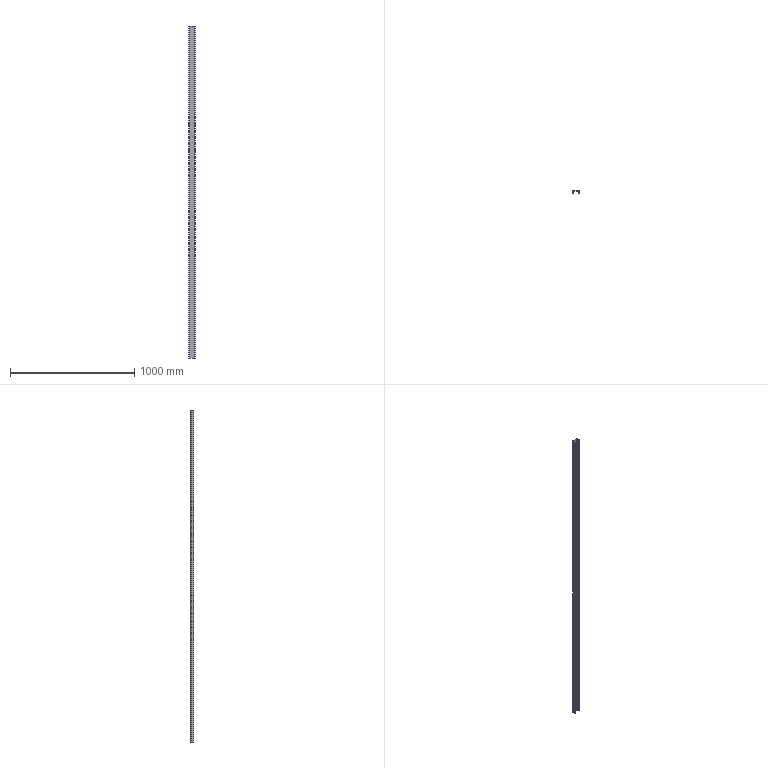Part | STEP file | VD-SYL0380DJ1006_1_2_1-6_STEP | 1 solid | 14 faces | box 50 x 25 x 2672 mm | volume 722540 mm3 | plane 10 | cylinder 4 | commonest cylinder face diameters 6 x2 12 x2
STEP:
#1=CARTESIAN_POINT('',(-19.,20.,1336.));
#2=VERTEX_POINT('',#1);
#3=CARTESIAN_POINT('',(-19.,20.,-1336.));
#4=VERTEX_POINT('',#3);
#5=CARTESIAN_POINT('',(-19.,20.,1336.));
#6=DIRECTION('',(0.,0.,-1.));
#7=VECTOR('',#6,1000.);
#8=LINE('',#5,#7);
#9=EDGE_CURVE('',#2,#4,#8,.T.);
#10=ORIENTED_EDGE('',*,*,#9,.T.);
#11=CARTESIAN_POINT('',(-25.,14.,-1336.));
#12=VERTEX_POINT('',#11);
#13=CARTESIAN_POINT('',(-19.,14.,-1336.));
#14=DIRECTION('',(0.,0.,-1.));
#15=DIRECTION('',(-1.,0.,0.));
#16=AXIS2_PLACEMENT_3D('',#13,#14,#15);
#17=CIRCLE('',#16,6.);
#18=EDGE_CURVE('',#12,#4,#17,.T.);
#19=ORIENTED_EDGE('',*,*,#18,.F.);
#20=CARTESIAN_POINT('',(-25.,14.,1336.));
#21=VERTEX_POINT('',#20);
#22=CARTESIAN_POINT('',(-25.,14.,-1336.));
#23=DIRECTION('',(0.,0.,1.));
#24=VECTOR('',#23,1000.);
#25=LINE('',#22,#24);
#26=EDGE_CURVE('',#12,#21,#25,.T.);
#27=ORIENTED_EDGE('',*,*,#26,.T.);
#28=CARTESIAN_POINT('',(-19.,14.,1336.));
#29=DIRECTION('',(0.,0.,1.));
#30=DIRECTION('',(0.,1.,0.));
#31=AXIS2_PLACEMENT_3D('',#28,#29,#30);
#32=CIRCLE('',#31,6.);
#33=EDGE_CURVE('',#2,#21,#32,.T.);
#34=ORIENTED_EDGE('',*,*,#33,.F.);
#35=EDGE_LOOP('',(#10,#19,#27,#34));
#36=FACE_OUTER_BOUND('',#35,.T.);
#37=CARTESIAN_POINT('',(-19.,14.,4819.219));
#38=DIRECTION('',(0.,0.,-1.));
#39=DIRECTION('',(-1.,0.,0.));
#40=AXIS2_PLACEMENT_3D('',#37,#38,#39);
#41=CYLINDRICAL_SURFACE('',#40,6.);
#42=ADVANCED_FACE('',(#36),#41,.T.);
#43=ORIENTED_EDGE('',*,*,#26,.F.);
#44=CARTESIAN_POINT('',(-25.,-5.,-1336.));
#45=VERTEX_POINT('',#44);
#46=CARTESIAN_POINT('',(-25.,-5.,-1336.));
#47=DIRECTION('',(0.,1.,0.));
#48=VECTOR('',#47,1000.);
#49=LINE('',#46,#48);
#50=EDGE_CURVE('',#45,#12,#49,.T.);
#51=ORIENTED_EDGE('',*,*,#50,.F.);
#52=CARTESIAN_POINT('',(-25.,-5.,1336.));
#53=VERTEX_POINT('',#52);
#54=CARTESIAN_POINT('',(-25.,-5.,1336.));
#55=DIRECTION('',(0.,0.,-1.));
#56=VECTOR('',#55,1000.);
#57=LINE('',#54,#56);
#58=EDGE_CURVE('',#53,#45,#57,.T.);
#59=ORIENTED_EDGE('',*,*,#58,.F.);
#60=CARTESIAN_POINT('',(-25.,14.,1336.));
#61=DIRECTION('',(0.,-1.,0.));
#62=VECTOR('',#61,1000.);
#63=LINE('',#60,#62);
#64=EDGE_CURVE('',#21,#53,#63,.T.);
#65=ORIENTED_EDGE('',*,*,#64,.F.);
#66=EDGE_LOOP('',(#43,#51,#59,#65));
#67=FACE_OUTER_BOUND('',#66,.T.);
#68=CARTESIAN_POINT('',(-25.,20.,-1336.));
#69=DIRECTION('',(-1.,0.,0.));
#70=DIRECTION('',(0.,0.,1.));
#71=AXIS2_PLACEMENT_3D('',#68,#69,#70);
#72=PLANE('',#71);
#73=ADVANCED_FACE('',(#67),#72,.T.);
#74=ORIENTED_EDGE('',*,*,#58,.T.);
#75=CARTESIAN_POINT('',(-22.,-5.,-1336.));
#76=VERTEX_POINT('',#75);
#77=CARTESIAN_POINT('',(-22.,-5.,-1336.));
#78=DIRECTION('',(-1.,0.,0.));
#79=VECTOR('',#78,1000.);
#80=LINE('',#77,#79);
#81=EDGE_CURVE('',#76,#45,#80,.T.);
#82=ORIENTED_EDGE('',*,*,#81,.F.);
#83=CARTESIAN_POINT('',(-22.,-5.,1336.));
#84=VERTEX_POINT('',#83);
#85=CARTESIAN_POINT('',(-22.,-5.,1336.));
#86=DIRECTION('',(0.,0.,-1.));
#87=VECTOR('',#86,1000.);
#88=LINE('',#85,#87);
#89=EDGE_CURVE('',#84,#76,#88,.T.);
#90=ORIENTED_EDGE('',*,*,#89,.F.);
#91=CARTESIAN_POINT('',(-25.,-5.,1336.));
#92=DIRECTION('',(1.,0.,0.));
#93=VECTOR('',#92,1000.);
#94=LINE('',#91,#93);
#95=EDGE_CURVE('',#53,#84,#94,.T.);
#96=ORIENTED_EDGE('',*,*,#95,.F.);
#97=EDGE_LOOP('',(#74,#82,#90,#96));
#98=FACE_OUTER_BOUND('',#97,.T.);
#99=CARTESIAN_POINT('',(-23.5,-5.,0.));
#100=DIRECTION('',(0.,-1.,0.));
#101=DIRECTION('',(0.,0.,-1.));
#102=AXIS2_PLACEMENT_3D('',#99,#100,#101);
#103=PLANE('',#102);
#104=ADVANCED_FACE('',(#98),#103,.T.);
#105=CARTESIAN_POINT('',(-22.,14.,-1336.));
#106=VERTEX_POINT('',#105);
#107=CARTESIAN_POINT('',(-22.,-5.,-1336.));
#108=DIRECTION('',(0.,1.,0.));
#109=VECTOR('',#108,1000.);
#110=LINE('',#107,#109);
#111=EDGE_CURVE('',#76,#106,#110,.T.);
#112=ORIENTED_EDGE('',*,*,#111,.T.);
#113=CARTESIAN_POINT('',(-22.,14.,1336.));
#114=VERTEX_POINT('',#113);
#115=CARTESIAN_POINT('',(-22.,14.,1336.));
#116=DIRECTION('',(0.,0.,-1.));
#117=VECTOR('',#116,1000.);
#118=LINE('',#115,#117);
#119=EDGE_CURVE('',#114,#106,#118,.T.);
#120=ORIENTED_EDGE('',*,*,#119,.F.);
#121=CARTESIAN_POINT('',(-22.,-5.,1336.));
#122=DIRECTION('',(0.,1.,0.));
#123=VECTOR('',#122,1000.);
#124=LINE('',#121,#123);
#125=EDGE_CURVE('',#84,#114,#124,.T.);
#126=ORIENTED_EDGE('',*,*,#125,.F.);
#127=ORIENTED_EDGE('',*,*,#89,.T.);
#128=EDGE_LOOP('',(#112,#120,#126,#127));
#129=FACE_OUTER_BOUND('',#128,.T.);
#130=CARTESIAN_POINT('',(-22.,20.,-1336.));
#131=DIRECTION('',(-1.,0.,0.));
#132=DIRECTION('',(0.,0.,1.));
#133=AXIS2_PLACEMENT_3D('',#130,#131,#132);
#134=PLANE('',#133);
#135=ADVANCED_FACE('',(#129),#134,.F.);
#136=CARTESIAN_POINT('',(-19.,17.,-1336.));
#137=VERTEX_POINT('',#136);
#138=CARTESIAN_POINT('',(-19.,14.,-1336.));
#139=DIRECTION('',(0.,0.,1.));
#140=DIRECTION('',(0.,1.,0.));
#141=AXIS2_PLACEMENT_3D('',#138,#139,#140);
#142=CIRCLE('',#141,3.);
#143=EDGE_CURVE('',#137,#106,#142,.T.);
#144=ORIENTED_EDGE('',*,*,#143,.F.);
#145=CARTESIAN_POINT('',(-19.,17.,1336.));
#146=VERTEX_POINT('',#145);
#147=CARTESIAN_POINT('',(-19.,17.,-1336.));
#148=DIRECTION('',(0.,0.,1.));
#149=VECTOR('',#148,1000.);
#150=LINE('',#147,#149);
#151=EDGE_CURVE('',#137,#146,#150,.T.);
#152=ORIENTED_EDGE('',*,*,#151,.T.);
#153=CARTESIAN_POINT('',(-19.,14.,1336.));
#154=DIRECTION('',(0.,0.,-1.));
#155=DIRECTION('',(-1.,0.,0.));
#156=AXIS2_PLACEMENT_3D('',#153,#154,#155);
#157=CIRCLE('',#156,3.);
#158=EDGE_CURVE('',#114,#146,#157,.T.);
#159=ORIENTED_EDGE('',*,*,#158,.F.);
#160=ORIENTED_EDGE('',*,*,#119,.T.);
#161=EDGE_LOOP('',(#144,#152,#159,#160));
#162=FACE_OUTER_BOUND('',#161,.T.);
#163=CARTESIAN_POINT('',(-19.,14.,4819.219));
#164=DIRECTION('',(0.,0.,-1.));
#165=DIRECTION('',(-1.,0.,0.));
#166=AXIS2_PLACEMENT_3D('',#163,#164,#165);
#167=CYLINDRICAL_SURFACE('',#166,3.);
#168=ADVANCED_FACE('',(#162),#167,.F.);
#169=CARTESIAN_POINT('',(25.,14.,1336.));
#170=VERTEX_POINT('',#169);
#171=CARTESIAN_POINT('',(25.,14.,-1336.));
#172=VERTEX_POINT('',#171);
#173=CARTESIAN_POINT('',(25.,14.,1336.));
#174=DIRECTION('',(0.,0.,-1.));
#175=VECTOR('',#174,1000.);
#176=LINE('',#173,#175);
#177=EDGE_CURVE('',#170,#172,#176,.T.);
#178=ORIENTED_EDGE('',*,*,#177,.F.);
#179=CARTESIAN_POINT('',(25.,-5.,1336.));
#180=VERTEX_POINT('',#179);
#181=CARTESIAN_POINT('',(25.,-5.,1336.));
#182=DIRECTION('',(0.,1.,0.));
#183=VECTOR('',#182,1000.);
#184=LINE('',#181,#183);
#185=EDGE_CURVE('',#180,#170,#184,.T.);
#186=ORIENTED_EDGE('',*,*,#185,.F.);
#187=CARTESIAN_POINT('',(25.,-5.,-1336.));
#188=VERTEX_POINT('',#187);
#189=CARTESIAN_POINT('',(25.,-5.,-1336.));
#190=DIRECTION('',(0.,0.,1.));
#191=VECTOR('',#190,1000.);
#192=LINE('',#189,#191);
#193=EDGE_CURVE('',#188,#180,#192,.T.);
#194=ORIENTED_EDGE('',*,*,#193,.F.);
#195=CARTESIAN_POINT('',(25.,14.,-1336.));
#196=DIRECTION('',(0.,-1.,0.));
#197=VECTOR('',#196,1000.);
#198=LINE('',#195,#197);
#199=EDGE_CURVE('',#172,#188,#198,.T.);
#200=ORIENTED_EDGE('',*,*,#199,.F.);
#201=EDGE_LOOP('',(#178,#186,#194,#200));
#202=FACE_OUTER_BOUND('',#201,.T.);
#203=CARTESIAN_POINT('',(25.,-5.,-1336.));
#204=DIRECTION('',(1.,0.,0.));
#205=DIRECTION('',(0.,1.,0.));
#206=AXIS2_PLACEMENT_3D('',#203,#204,#205);
#207=PLANE('',#206);
#208=ADVANCED_FACE('',(#202),#207,.T.);
#209=CARTESIAN_POINT('',(22.,-5.,-1336.));
#210=VERTEX_POINT('',#209);
#211=CARTESIAN_POINT('',(22.,-5.,-1336.));
#212=DIRECTION('',(1.,0.,0.));
#213=VECTOR('',#212,1000.);
#214=LINE('',#211,#213);
#215=EDGE_CURVE('',#210,#188,#214,.T.);
#216=ORIENTED_EDGE('',*,*,#215,.T.);
#217=ORIENTED_EDGE('',*,*,#193,.T.);
#218=CARTESIAN_POINT('',(22.,-5.,1336.));
#219=VERTEX_POINT('',#218);
#220=CARTESIAN_POINT('',(25.,-5.,1336.));
#221=DIRECTION('',(-1.,0.,0.));
#222=VECTOR('',#221,1000.);
#223=LINE('',#220,#222);
#224=EDGE_CURVE('',#180,#219,#223,.T.);
#225=ORIENTED_EDGE('',*,*,#224,.T.);
#226=CARTESIAN_POINT('',(22.,-5.,1336.));
#227=DIRECTION('',(0.,0.,-1.));
#228=VECTOR('',#227,1000.);
#229=LINE('',#226,#228);
#230=EDGE_CURVE('',#219,#210,#229,.T.);
#231=ORIENTED_EDGE('',*,*,#230,.T.);
#232=EDGE_LOOP('',(#216,#217,#225,#231));
#233=FACE_OUTER_BOUND('',#232,.T.);
#234=CARTESIAN_POINT('',(23.5,-5.,0.));
#235=DIRECTION('',(0.,1.,0.));
#236=DIRECTION('',(1.,0.,0.));
#237=AXIS2_PLACEMENT_3D('',#234,#235,#236);
#238=PLANE('',#237);
#239=ADVANCED_FACE('',(#233),#238,.F.);
#240=CARTESIAN_POINT('',(22.,14.,1336.));
#241=VERTEX_POINT('',#240);
#242=CARTESIAN_POINT('',(22.,14.,1336.));
#243=DIRECTION('',(0.,-1.,0.));
#244=VECTOR('',#243,1000.);
#245=LINE('',#242,#244);
#246=EDGE_CURVE('',#241,#219,#245,.T.);
#247=ORIENTED_EDGE('',*,*,#246,.F.);
#248=CARTESIAN_POINT('',(22.,14.,-1336.));
#249=VERTEX_POINT('',#248);
#250=CARTESIAN_POINT('',(22.,14.,-1336.));
#251=DIRECTION('',(0.,0.,1.));
#252=VECTOR('',#251,1000.);
#253=LINE('',#250,#252);
#254=EDGE_CURVE('',#249,#241,#253,.T.);
#255=ORIENTED_EDGE('',*,*,#254,.F.);
#256=CARTESIAN_POINT('',(22.,14.,-1336.));
#257=DIRECTION('',(0.,-1.,0.));
#258=VECTOR('',#257,1000.);
#259=LINE('',#256,#258);
#260=EDGE_CURVE('',#249,#210,#259,.T.);
#261=ORIENTED_EDGE('',*,*,#260,.T.);
#262=ORIENTED_EDGE('',*,*,#230,.F.);
#263=EDGE_LOOP('',(#247,#255,#261,#262));
#264=FACE_OUTER_BOUND('',#263,.T.);
#265=CARTESIAN_POINT('',(22.,-5.,-1336.));
#266=DIRECTION('',(1.,0.,0.));
#267=DIRECTION('',(0.,1.,0.));
#268=AXIS2_PLACEMENT_3D('',#265,#266,#267);
#269=PLANE('',#268);
#270=ADVANCED_FACE('',(#264),#269,.F.);
#271=CARTESIAN_POINT('',(19.,17.,-1336.));
#272=VERTEX_POINT('',#271);
#273=CARTESIAN_POINT('',(19.,14.,-1336.));
#274=DIRECTION('',(0.,0.,1.));
#275=DIRECTION('',(1.,0.,0.));
#276=AXIS2_PLACEMENT_3D('',#273,#274,#275);
#277=CIRCLE('',#276,3.);
#278=EDGE_CURVE('',#249,#272,#277,.T.);
#279=ORIENTED_EDGE('',*,*,#278,.F.);
#280=ORIENTED_EDGE('',*,*,#254,.T.);
#281=CARTESIAN_POINT('',(19.,17.,1336.));
#282=VERTEX_POINT('',#281);
#283=CARTESIAN_POINT('',(19.,14.,1336.));
#284=DIRECTION('',(0.,0.,-1.));
#285=DIRECTION('',(0.,1.,0.));
#286=AXIS2_PLACEMENT_3D('',#283,#284,#285);
#287=CIRCLE('',#286,3.);
#288=EDGE_CURVE('',#282,#241,#287,.T.);
#289=ORIENTED_EDGE('',*,*,#288,.F.);
#290=CARTESIAN_POINT('',(19.,17.,1336.));
#291=DIRECTION('',(0.,0.,-1.));
#292=VECTOR('',#291,1000.);
#293=LINE('',#290,#292);
#294=EDGE_CURVE('',#282,#272,#293,.T.);
#295=ORIENTED_EDGE('',*,*,#294,.T.);
#296=EDGE_LOOP('',(#279,#280,#289,#295));
#297=FACE_OUTER_BOUND('',#296,.T.);
#298=CARTESIAN_POINT('',(19.,14.,4819.219));
#299=DIRECTION('',(0.,0.,-1.));
#300=DIRECTION('',(-1.,0.,0.));
#301=AXIS2_PLACEMENT_3D('',#298,#299,#300);
#302=CYLINDRICAL_SURFACE('',#301,3.);
#303=ADVANCED_FACE('',(#297),#302,.F.);
#304=CARTESIAN_POINT('',(-19.,17.,1336.));
#305=DIRECTION('',(1.,0.,0.));
#306=VECTOR('',#305,1000.);
#307=LINE('',#304,#306);
#308=EDGE_CURVE('',#146,#282,#307,.T.);
#309=ORIENTED_EDGE('',*,*,#308,.F.);
#310=ORIENTED_EDGE('',*,*,#151,.F.);
#311=CARTESIAN_POINT('',(-19.,17.,-1336.));
#312=DIRECTION('',(1.,0.,0.));
#313=VECTOR('',#312,1000.);
#314=LINE('',#311,#313);
#315=EDGE_CURVE('',#137,#272,#314,.T.);
#316=ORIENTED_EDGE('',*,*,#315,.T.);
#317=ORIENTED_EDGE('',*,*,#294,.F.);
#318=EDGE_LOOP('',(#309,#310,#316,#317));
#319=FACE_OUTER_BOUND('',#318,.T.);
#320=CARTESIAN_POINT('',(25.,17.,-1336.));
#321=DIRECTION('',(0.,1.,0.));
#322=DIRECTION('',(1.,0.,0.));
#323=AXIS2_PLACEMENT_3D('',#320,#321,#322);
#324=PLANE('',#323);
#325=ADVANCED_FACE('',(#319),#324,.F.);
#326=ORIENTED_EDGE('',*,*,#143,.T.);
#327=ORIENTED_EDGE('',*,*,#111,.F.);
#328=ORIENTED_EDGE('',*,*,#81,.T.);
#329=ORIENTED_EDGE('',*,*,#50,.T.);
#330=ORIENTED_EDGE('',*,*,#18,.T.);
#331=CARTESIAN_POINT('',(19.,20.,-1336.));
#332=VERTEX_POINT('',#331);
#333=CARTESIAN_POINT('',(-19.,20.,-1336.));
#334=DIRECTION('',(1.,0.,0.));
#335=VECTOR('',#334,1000.);
#336=LINE('',#333,#335);
#337=EDGE_CURVE('',#4,#332,#336,.T.);
#338=ORIENTED_EDGE('',*,*,#337,.T.);
#339=CARTESIAN_POINT('',(19.,14.,-1336.));
#340=DIRECTION('',(0.,0.,-1.));
#341=DIRECTION('',(0.,1.,0.));
#342=AXIS2_PLACEMENT_3D('',#339,#340,#341);
#343=CIRCLE('',#342,6.);
#344=EDGE_CURVE('',#332,#172,#343,.T.);
#345=ORIENTED_EDGE('',*,*,#344,.T.);
#346=ORIENTED_EDGE('',*,*,#199,.T.);
#347=ORIENTED_EDGE('',*,*,#215,.F.);
#348=ORIENTED_EDGE('',*,*,#260,.F.);
#349=ORIENTED_EDGE('',*,*,#278,.T.);
#350=ORIENTED_EDGE('',*,*,#315,.F.);
#351=EDGE_LOOP('',(#326,#327,#328,#329,#330,#338,#345,#346,#347,#348,#349,#350));
#352=FACE_OUTER_BOUND('',#351,.T.);
#353=CARTESIAN_POINT('',(0.,18.5,-1336.));
#354=DIRECTION('',(0.,0.,-1.));
#355=DIRECTION('',(0.,-1.,0.));
#356=AXIS2_PLACEMENT_3D('',#353,#354,#355);
#357=PLANE('',#356);
#358=ADVANCED_FACE('',(#352),#357,.T.);
#359=ORIENTED_EDGE('',*,*,#9,.F.);
#360=CARTESIAN_POINT('',(19.,20.,1336.));
#361=VERTEX_POINT('',#360);
#362=CARTESIAN_POINT('',(19.,20.,1336.));
#363=DIRECTION('',(-1.,0.,0.));
#364=VECTOR('',#363,1000.);
#365=LINE('',#362,#364);
#366=EDGE_CURVE('',#361,#2,#365,.T.);
#367=ORIENTED_EDGE('',*,*,#366,.F.);
#368=CARTESIAN_POINT('',(19.,20.,-1336.));
#369=DIRECTION('',(0.,0.,1.));
#370=VECTOR('',#369,1000.);
#371=LINE('',#368,#370);
#372=EDGE_CURVE('',#332,#361,#371,.T.);
#373=ORIENTED_EDGE('',*,*,#372,.F.);
#374=ORIENTED_EDGE('',*,*,#337,.F.);
#375=EDGE_LOOP('',(#359,#367,#373,#374));
#376=FACE_OUTER_BOUND('',#375,.T.);
#377=CARTESIAN_POINT('',(25.,20.,-1336.));
#378=DIRECTION('',(0.,1.,0.));
#379=DIRECTION('',(1.,0.,0.));
#380=AXIS2_PLACEMENT_3D('',#377,#378,#379);
#381=PLANE('',#380);
#382=ADVANCED_FACE('',(#376),#381,.T.);
#383=ORIENTED_EDGE('',*,*,#33,.T.);
#384=ORIENTED_EDGE('',*,*,#64,.T.);
#385=ORIENTED_EDGE('',*,*,#95,.T.);
#386=ORIENTED_EDGE('',*,*,#125,.T.);
#387=ORIENTED_EDGE('',*,*,#158,.T.);
#388=ORIENTED_EDGE('',*,*,#308,.T.);
#389=ORIENTED_EDGE('',*,*,#288,.T.);
#390=ORIENTED_EDGE('',*,*,#246,.T.);
#391=ORIENTED_EDGE('',*,*,#224,.F.);
#392=ORIENTED_EDGE('',*,*,#185,.T.);
#393=CARTESIAN_POINT('',(19.,14.,1336.));
#394=DIRECTION('',(0.,0.,1.));
#395=DIRECTION('',(1.,0.,0.));
#396=AXIS2_PLACEMENT_3D('',#393,#394,#395);
#397=CIRCLE('',#396,6.);
#398=EDGE_CURVE('',#170,#361,#397,.T.);
#399=ORIENTED_EDGE('',*,*,#398,.T.);
#400=ORIENTED_EDGE('',*,*,#366,.T.);
#401=EDGE_LOOP('',(#383,#384,#385,#386,#387,#388,#389,#390,#391,#392,#399,#400));
#402=FACE_OUTER_BOUND('',#401,.T.);
#403=CARTESIAN_POINT('',(0.,18.5,1336.));
#404=DIRECTION('',(0.,0.,-1.));
#405=DIRECTION('',(0.,-1.,0.));
#406=AXIS2_PLACEMENT_3D('',#403,#404,#405);
#407=PLANE('',#406);
#408=ADVANCED_FACE('',(#402),#407,.F.);
#409=ORIENTED_EDGE('',*,*,#177,.T.);
#410=ORIENTED_EDGE('',*,*,#344,.F.);
#411=ORIENTED_EDGE('',*,*,#372,.T.);
#412=ORIENTED_EDGE('',*,*,#398,.F.);
#413=EDGE_LOOP('',(#409,#410,#411,#412));
#414=FACE_OUTER_BOUND('',#413,.T.);
#415=CARTESIAN_POINT('',(19.,14.,4819.219));
#416=DIRECTION('',(0.,0.,-1.));
#417=DIRECTION('',(-1.,0.,0.));
#418=AXIS2_PLACEMENT_3D('',#415,#416,#417);
#419=CYLINDRICAL_SURFACE('',#418,6.);
#420=ADVANCED_FACE('',(#414),#419,.T.);
#421=CLOSED_SHELL('',(#42,#73,#104,#135,#168,#208,#239,#270,#303,#325,#358,#382,#408,#420));
#422=MANIFOLD_SOLID_BREP('',#421);
#423=CARTESIAN_POINT('',(0.,0.,0.));
#424=DIRECTION('',(0.,0.,1.));
#425=DIRECTION('',(1.,0.,0.));
#426=AXIS2_PLACEMENT_3D('',#423,#424,#425);
#427=(LENGTH_UNIT()NAMED_UNIT(*)SI_UNIT(.MILLI.,.METRE.));
#428=UNCERTAINTY_MEASURE_WITH_UNIT(LENGTH_MEASURE(0.00001),#427,'','');
#429=(NAMED_UNIT(*)PLANE_ANGLE_UNIT()SI_UNIT($,.RADIAN.));
#430=(NAMED_UNIT(*)SI_UNIT($,.STERADIAN.)SOLID_ANGLE_UNIT());
#431=(GEOMETRIC_REPRESENTATION_CONTEXT(3)GLOBAL_UNCERTAINTY_ASSIGNED_CONTEXT((#428))GLOBAL_UNIT_ASSIGNED_CONTEXT((#427,#429,#430))REPRESENTATION_CONTEXT('',''));
#432=ADVANCED_BREP_SHAPE_REPRESENTATION('',(#422,#426),#431);